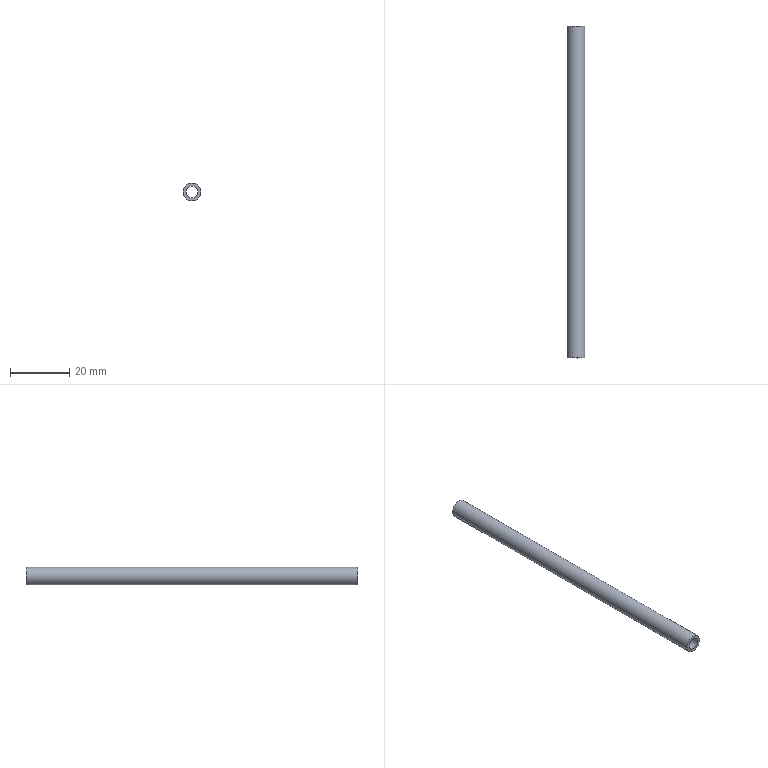Part | NX | features solid 2 | 1 solid | 4 faces | box 6 x 111.613 x 6 mm | volume 1753 mm3 | cylinder 2 | plane 2 | commonest cylinder face diameters 4 x1 6 x1
STEP:
#1=CARTESIAN_POINT('',(474.,85.,347.));
#2=VERTEX_POINT('',#1);
#3=CARTESIAN_POINT('',(472.,85.,347.));
#4=DIRECTION('',(0.,-1.,0.));
#5=DIRECTION('',(1.,0.,0.));
#6=AXIS2_PLACEMENT_3D('',#3,#4,#5);
#7=CIRCLE('',#6,2.);
#8=EDGE_CURVE('',#2,#2,#7,.T.);
#9=ORIENTED_EDGE('',*,*,#8,.F.);
#10=EDGE_LOOP('',(#9));
#11=FACE_BOUND('',#10,.T.);
#12=CARTESIAN_POINT('',(474.,-26.613,347.));
#13=VERTEX_POINT('',#12);
#14=CARTESIAN_POINT('',(472.,-26.613,347.));
#15=DIRECTION('',(0.,-1.,0.));
#16=DIRECTION('',(1.,0.,0.));
#17=AXIS2_PLACEMENT_3D('',#14,#15,#16);
#18=CIRCLE('',#17,2.);
#19=EDGE_CURVE('',#13,#13,#18,.T.);
#20=ORIENTED_EDGE('',*,*,#19,.T.);
#21=EDGE_LOOP('',(#20));
#22=FACE_BOUND('',#21,.T.);
#23=CARTESIAN_POINT('',(472.,-193.824,347.));
#24=DIRECTION('',(0.,1.,0.));
#25=DIRECTION('',(-1.,0.,0.));
#26=AXIS2_PLACEMENT_3D('',#23,#24,#25);
#27=CYLINDRICAL_SURFACE('',#26,2.);
#28=ADVANCED_FACE('',(#11,#22),#27,.F.);
#29=CARTESIAN_POINT('',(475.,85.,347.));
#30=VERTEX_POINT('',#29);
#31=CARTESIAN_POINT('',(472.,85.,347.));
#32=DIRECTION('',(0.,-1.,0.));
#33=DIRECTION('',(1.,0.,0.));
#34=AXIS2_PLACEMENT_3D('',#31,#32,#33);
#35=CIRCLE('',#34,3.);
#36=EDGE_CURVE('',#30,#30,#35,.T.);
#37=ORIENTED_EDGE('',*,*,#36,.T.);
#38=EDGE_LOOP('',(#37));
#39=FACE_BOUND('',#38,.T.);
#40=CARTESIAN_POINT('',(475.,-26.613,347.));
#41=VERTEX_POINT('',#40);
#42=CARTESIAN_POINT('',(472.,-26.613,347.));
#43=DIRECTION('',(0.,-1.,0.));
#44=DIRECTION('',(1.,0.,0.));
#45=AXIS2_PLACEMENT_3D('',#42,#43,#44);
#46=CIRCLE('',#45,3.);
#47=EDGE_CURVE('',#41,#41,#46,.T.);
#48=ORIENTED_EDGE('',*,*,#47,.F.);
#49=EDGE_LOOP('',(#48));
#50=FACE_BOUND('',#49,.T.);
#51=CARTESIAN_POINT('',(472.,-193.824,347.));
#52=DIRECTION('',(0.,1.,0.));
#53=DIRECTION('',(-1.,0.,0.));
#54=AXIS2_PLACEMENT_3D('',#51,#52,#53);
#55=CYLINDRICAL_SURFACE('',#54,3.);
#56=ADVANCED_FACE('',(#39,#50),#55,.T.);
#57=ORIENTED_EDGE('',*,*,#8,.T.);
#58=EDGE_LOOP('',(#57));
#59=FACE_BOUND('',#58,.T.);
#60=ORIENTED_EDGE('',*,*,#36,.F.);
#61=EDGE_LOOP('',(#60));
#62=FACE_BOUND('',#61,.T.);
#63=CARTESIAN_POINT('',(472.,85.,347.));
#64=DIRECTION('',(0.,-1.,0.));
#65=DIRECTION('',(1.,0.,0.));
#66=AXIS2_PLACEMENT_3D('',#63,#64,#65);
#67=PLANE('',#66);
#68=ADVANCED_FACE('',(#59,#62),#67,.F.);
#69=ORIENTED_EDGE('',*,*,#19,.F.);
#70=EDGE_LOOP('',(#69));
#71=FACE_BOUND('',#70,.T.);
#72=ORIENTED_EDGE('',*,*,#47,.T.);
#73=EDGE_LOOP('',(#72));
#74=FACE_BOUND('',#73,.T.);
#75=CARTESIAN_POINT('',(456.131,-26.613,203.));
#76=DIRECTION('',(0.,-1.,0.));
#77=DIRECTION('',(1.,0.,0.));
#78=AXIS2_PLACEMENT_3D('',#75,#76,#77);
#79=PLANE('',#78);
#80=ADVANCED_FACE('',(#71,#74),#79,.T.);
#81=CLOSED_SHELL('',(#28,#56,#68,#80));
#82=MANIFOLD_SOLID_BREP('',#81);
#83=(LENGTH_UNIT()NAMED_UNIT(*)SI_UNIT(.MILLI.,.METRE.));
#84=UNCERTAINTY_MEASURE_WITH_UNIT(LENGTH_MEASURE(0.00001),#83,'','');
#85=(NAMED_UNIT(*)PLANE_ANGLE_UNIT()SI_UNIT($,.RADIAN.));
#86=(NAMED_UNIT(*)SI_UNIT($,.STERADIAN.)SOLID_ANGLE_UNIT());
#87=(GEOMETRIC_REPRESENTATION_CONTEXT(3)GLOBAL_UNCERTAINTY_ASSIGNED_CONTEXT((#84))GLOBAL_UNIT_ASSIGNED_CONTEXT((#83,#85,#86))REPRESENTATION_CONTEXT('',''));
#88=ADVANCED_BREP_SHAPE_REPRESENTATION('',(#82),#87);